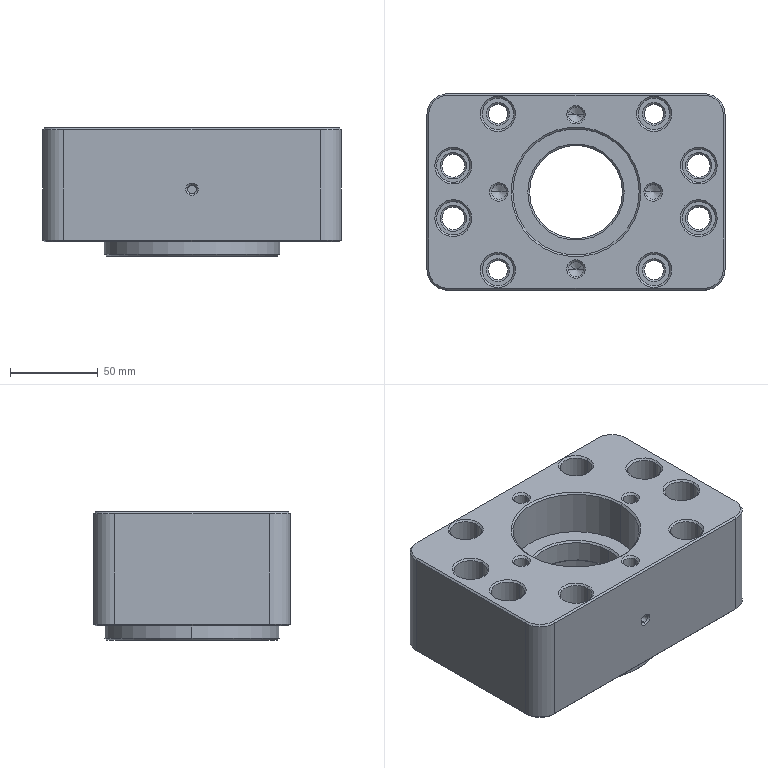NC program | NX | posted with a generic post | part box 170 x 112 x 73 mm
Lines 2870 to 3892 of 12198:
(ZLEVEL_PROFILE , TOOL : D26)
N5690 T16 M6
N5692 G54
N5694 G17 G0 G90 X100.366 Y-39.31 S1700 M3
N5696 G43 Z30. H16
N5698 Z-0.349
N5700 G94 G1 X99.295 Y-39.929 F1000.
N5702 G3 X97.997 Y-42.182 R2.6
N5704 G1 X97.998 Y-43.259 F1700.
N5706 X97.999 Y-44.01
N5708 G2 X97.948 Y-45.558 R44.459
N5710 X97.732 Y-47.632 R28.441
N5712 X97.189 Y-50.339 R30.228
N5714 X95.838 Y-54.175 R27.501
N5716 X92.835 Y-59.228 R26.139
N5718 X90.04 Y-62.3 R28.22
N5720 X88.018 Y-63.983 R28.318
N5722 X86.327 Y-65.148 R28.811
N5724 X83.495 Y-66.697 R27.897
N5726 X81.085 Y-67.653 R30.882
N5728 X77.976 Y-68.509 R29.143
N5730 X75.343 Y-68.886 R30.526
N5732 X73.425 Y-68.993 R29.282
N5734 G1 X73.01 Y-68.999
N5736 X72.259 Y-68.997
N5738 X71.182
N5740 G3 X68.93 Y-70.296 R2.6
N5742 G1 X68.311 Y-71.366
N5744 G0 Z30.
N5746 X100.367 Y-39.309
N5748 Z-0.699
N5750 G1 X99.295 Y-39.929 F1000.
N5752 G3 X97.997 Y-42.182 R2.6
N5754 G1 X97.998 Y-43.259 F1700.
N5756 X97.999 Y-44.01
N5758 G2 X97.948 Y-45.558 R41.97
N5760 X97.732 Y-47.632 R28.038
N5762 X97.183 Y-50.359 R29.625
N5764 X95.831 Y-54.19 R27.273
N5766 X94.533 Y-56.694 R26.82
N5768 X92.811 Y-59.258 R28.325
N5770 X90.033 Y-62.306 R28.036
N5772 X88.018 Y-63.983 R28.19
N5774 X86.328 Y-65.148 R28.641
N5776 X84.741 Y-66.068 R29.677
N5778 X82.981 Y-66.917 R27.561
N5780 X81.085 Y-67.653 R27.854
N5782 X77.947 Y-68.514 R28.668
N5784 X75.343 Y-68.886 R30.089
N5786 X73.425 Y-68.993 R28.844
N5788 G1 X73.01 Y-68.999
N5790 X72.259 Y-68.998
N5792 X71.182 Y-68.997
N5794 G3 X68.93 Y-70.296 R2.6
N5796 G1 X68.31 Y-71.367
N5798 G0 Z30.
N5800 X100.6 Y-39.169
N5802 Z-1.048
N5804 G1 X99.292 Y-39.928 F1000.
N5806 G3 X97.997 Y-42.182 R2.6
N5808 G1 X98. Y-43.617 F1700.
N5810 Y-44.
N5812 G2 X72.986 Y-69. R25.
N5814 G1 X72.617
N5816 X71.182 Y-68.997
N5818 G3 X68.928 Y-70.292 R2.6
N5820 G1 X68.169 Y-71.6
N5822 G0 Z30.
N5824 X100.6 Y-39.169
N5826 Z-1.398
N5828 G1 X99.292 Y-39.928 F1000.
N5830 G3 X97.997 Y-42.182 R2.6
N5832 G1 X98. Y-43.617 F1700.
N5834 Y-44.
N5836 G2 X72.986 Y-69. R25.
N5838 G1 X72.617
N5840 X71.182 Y-68.997
N5842 G3 X68.928 Y-70.292 R2.6
N5844 G1 X68.169 Y-71.6
N5846 G0 Z30.
N5848 X100.6 Y-39.169
N5850 Z-1.747
N5852 G1 X99.292 Y-39.928 F1000.
N5854 G3 X97.997 Y-42.182 R2.6
N5856 G1 X98. Y-43.617 F1700.
N5858 Y-44.
N5860 G2 X72.986 Y-69. R25.
N5862 G1 X72.617
N5864 X71.182 Y-68.997
N5866 G3 X68.928 Y-70.292 R2.6
N5868 G1 X68.169 Y-71.6
N5870 G0 Z30.
N5872 X100.6 Y-39.169
N5874 Z-2.097
N5876 G1 X99.292 Y-39.928 F1000.
N5878 G3 X97.997 Y-42.182 R2.6
N5880 G1 X98. Y-43.617 F1700.
N5882 Y-44.
N5884 G2 X72.986 Y-69. R25.
N5886 G1 X72.617
N5888 X71.182 Y-68.997
N5890 G3 X68.928 Y-70.292 R2.6
N5892 G1 X68.169 Y-71.6
N5894 G0 Z30.
N5896 X100.6 Y-39.169
N5898 Z-2.446
N5900 G1 X99.292 Y-39.928 F1000.
N5902 G3 X97.997 Y-42.182 R2.6
N5904 G1 X98. Y-43.617 F1700.
N5906 Y-44.
N5908 G2 X72.986 Y-69. R25.
N5910 G1 X72.617
N5912 X71.182 Y-68.997
N5914 G3 X68.928 Y-70.292 R2.6
N5916 G1 X68.169 Y-71.6
N5918 G0 Z30.
N5920 X100.6 Y-39.169
N5922 Z-2.796
N5924 G1 X99.292 Y-39.928 F1000.
N5926 G3 X97.997 Y-42.182 R2.6
N5928 G1 X98. Y-43.617 F1700.
N5930 Y-44.
N5932 G2 X72.986 Y-69. R25.
N5934 G1 X72.617
N5936 X71.182 Y-68.997
N5938 G3 X68.928 Y-70.292 R2.6
N5940 G1 X68.169 Y-71.6
N5942 G0 Z30.
N5944 X100.6 Y-39.169
N5946 Z-3.145
N5948 G1 X99.293 Y-39.928 F1000.
N5950 G3 X97.997 Y-42.182 R2.6
N5952 G1 X98. Y-43.617 F1700.
N5954 Y-44.
N5956 G2 X72.986 Y-69. R25.
N5958 G1 X72.617
N5960 X71.182 Y-68.997
N5962 G3 X68.928 Y-70.292 R2.6
N5964 G1 X68.169 Y-71.6
N5966 G0 Z30.
N5968 X100.6 Y-39.169
N5970 Z-3.495
N5972 G1 X99.293 Y-39.928 F1000.
N5974 G3 X97.997 Y-42.182 R2.6
N5976 G1 X98. Y-43.617 F1700.
N5978 Y-44.
N5980 G2 X72.986 Y-69. R25.
N5982 G1 X72.617
N5984 X71.182 Y-68.997
N5986 G3 X68.928 Y-70.292 R2.6
N5988 G1 X68.169 Y-71.6
N5990 G0 Z30.
N5992 X100.6 Y-39.17
N5994 Z-3.844
N5996 G1 X99.293 Y-39.928 F1000.
N5998 G3 X97.997 Y-42.182 R2.6
N6000 G1 X98. Y-43.617 F1700.
N6002 Y-44.
N6004 G2 X72.986 Y-69. R25.
N6006 G1 X72.617
N6008 X71.182 Y-68.997
N6010 G3 X68.928 Y-70.292 R2.6
N6012 G1 X68.169 Y-71.6
N6014 G0 Z30.
N6016 X100.6 Y-39.17
N6018 Z-4.194
N6020 G1 X99.293 Y-39.928 F1000.
N6022 G3 X97.997 Y-42.182 R2.6
N6024 G1 X98. Y-43.617 F1700.
N6026 Y-44.
N6028 G2 X72.986 Y-69. R25.
N6030 G1 X72.617
N6032 X71.182 Y-68.997
N6034 G3 X68.928 Y-70.292 R2.6
N6036 G1 X68.169 Y-71.6
N6038 G0 Z30.
N6040 X100.6 Y-39.17
N6042 Z-4.543
N6044 G1 X99.293 Y-39.928 F1000.
N6046 G3 X97.997 Y-42.182 R2.6
N6048 G1 X98. Y-43.617 F1700.
N6050 Y-44.
N6052 G2 X72.986 Y-69. R25.
N6054 G1 X72.617
N6056 X71.182 Y-68.997
N6058 G3 X68.928 Y-70.292 R2.6
N6060 G1 X68.169 Y-71.6
N6062 G0 Z30.
N6064 X100.6 Y-39.17
N6066 Z-4.892
N6068 G1 X99.293 Y-39.928 F1000.
N6070 G3 X97.997 Y-42.182 R2.6
N6072 G1 X98. Y-43.617 F1700.
N6074 Y-44.
N6076 G2 X72.986 Y-69. R25.
N6078 G1 X72.617
N6080 X71.182 Y-68.997
N6082 G3 X68.928 Y-70.292 R2.6
N6084 G1 X68.169 Y-71.6
N6086 G0 Z30.
N6088 X100.6 Y-39.17
N6090 Z-5.242
N6092 G1 X99.293 Y-39.928 F1000.
N6094 G3 X97.997 Y-42.182 R2.6
N6096 G1 X98. Y-43.617 F1700.
N6098 Y-44.
N6100 G2 X72.986 Y-69. R25.
N6102 G1 X72.617
N6104 X71.182 Y-68.997
N6106 G3 X68.928 Y-70.292 R2.6
N6108 G1 X68.169 Y-71.6
N6110 G0 Z30.
N6112 X100.6 Y-39.17
N6114 Z-5.591
N6116 G1 X99.293 Y-39.928 F1000.
N6118 G3 X97.997 Y-42.182 R2.6
N6120 G1 X98. Y-43.617 F1700.
N6122 Y-44.
N6124 G2 X72.986 Y-69. R25.
N6126 G1 X72.617
N6128 X71.182 Y-68.997
N6130 G3 X68.928 Y-70.292 R2.6
N6132 G1 X68.169 Y-71.6
N6134 G0 Z30.
N6136 X100.6 Y-39.17
N6138 Z-5.941
N6140 G1 X99.293 Y-39.928 F1000.
N6142 G3 X97.997 Y-42.182 R2.6
N6144 G1 X98. Y-43.617 F1700.
N6146 Y-44.
N6148 G2 X72.986 Y-69. R25.
N6150 G1 X72.617
N6152 X71.182 Y-68.997
N6154 G3 X68.928 Y-70.292 R2.6
N6156 G1 X68.169 Y-71.6
N6158 G0 Z30.
N6160 X100.6 Y-39.17
N6162 Z-6.29
N6164 G1 X99.293 Y-39.928 F1000.
N6166 G3 X97.997 Y-42.182 R2.6
N6168 G1 X98. Y-43.617 F1700.
N6170 Y-44.
N6172 G2 X72.986 Y-69. R25.
N6174 G1 X72.617
N6176 X71.182 Y-68.997
N6178 G3 X68.928 Y-70.293 R2.6
N6180 G1 X68.169 Y-71.6
N6182 G0 Z30.
N6184 X100.6 Y-39.17
N6186 Z-6.64
N6188 G1 X99.293 Y-39.928 F1000.
N6190 G3 X97.997 Y-42.182 R2.6
N6192 G1 X98. Y-43.617 F1700.
N6194 Y-44.
N6196 G2 X72.986 Y-69. R25.
N6198 G1 X72.617
N6200 X71.182 Y-68.997
N6202 G3 X68.928 Y-70.293 R2.6
N6204 G1 X68.169 Y-71.6
N6206 G0 Z30.
N6208 X100.6 Y-39.17
N6210 Z-6.989
N6212 G1 X99.293 Y-39.928 F1000.
N6214 G3 X97.997 Y-42.182 R2.6
N6216 G1 X98. Y-43.617 F1700.
N6218 Y-44.
N6220 G2 X72.986 Y-69. R25.
N6222 G1 X72.617
N6224 X71.182 Y-68.997
N6226 G3 X68.928 Y-70.293 R2.6
N6228 G1 X68.169 Y-71.6
N6230 G0 Z30.
N6232 X100.6 Y-39.17
N6234 Z-7.339
N6236 G1 X99.293 Y-39.928 F1000.
N6238 G3 X97.997 Y-42.182 R2.6
N6240 G1 X98. Y-43.617 F1700.
N6242 Y-44.
N6244 G2 X72.986 Y-69. R25.
N6246 G1 X72.617
N6248 X71.182 Y-68.997
N6250 G3 X68.928 Y-70.293 R2.6
N6252 G1 X68.169 Y-71.6
N6254 G0 Z30.
N6256 X100.6 Y-39.17
N6258 Z-7.688
N6260 G1 X99.293 Y-39.928 F1000.
N6262 G3 X97.997 Y-42.182 R2.6
N6264 G1 X98. Y-43.617 F1700.
N6266 Y-44.
N6268 G2 X72.986 Y-69. R25.
N6270 G1 X72.617
N6272 X71.182 Y-68.997
N6274 G3 X68.928 Y-70.293 R2.6
N6276 G1 X68.17 Y-71.6
N6278 G0 Z30.
N6280 X100.6 Y-39.17
N6282 Z-8.038
N6284 G1 X99.293 Y-39.928 F1000.
N6286 G3 X97.997 Y-42.182 R2.6
N6288 G1 X98. Y-43.617 F1700.
N6290 Y-44.
N6292 G2 X72.986 Y-69. R25.
N6294 G1 X72.617
N6296 X71.182 Y-68.997
N6298 G3 X68.928 Y-70.293 R2.6
N6300 G1 X68.17 Y-71.6
N6302 G0 Z30.
N6304 X100.6 Y-39.17
N6306 Z-8.387
N6308 G1 X99.293 Y-39.928 F1000.
N6310 G3 X97.997 Y-42.182 R2.6
N6312 G1 X98. Y-43.617 F1700.
N6314 Y-44.
N6316 G2 X72.986 Y-69. R25.
N6318 G1 X72.617
N6320 X71.182 Y-68.997
N6322 G3 X68.928 Y-70.293 R2.6
N6324 G1 X68.17 Y-71.6
N6326 G0 Z30.
N6328 X100.6 Y-39.17
N6330 Z-8.737
N6332 G1 X99.293 Y-39.928 F1000.
N6334 G3 X97.997 Y-42.182 R2.6
N6336 G1 X98. Y-43.617 F1700.
N6338 Y-44.
N6340 G2 X72.986 Y-69. R25.
N6342 G1 X72.617
N6344 X71.182 Y-68.997
N6346 G3 X68.928 Y-70.293 R2.6
N6348 G1 X68.17 Y-71.6
N6350 G0 Z30.
N6352 X100.6 Y-39.17
N6354 Z-9.086
N6356 G1 X99.293 Y-39.928 F1000.
N6358 G3 X97.997 Y-42.182 R2.6
N6360 G1 X98. Y-43.617 F1700.
N6362 Y-44.
N6364 G2 X72.986 Y-69. R25.
N6366 G1 X72.617
N6368 X71.182 Y-68.997
N6370 G3 X68.928 Y-70.293 R2.6
N6372 G1 X68.17 Y-71.6
N6374 G0 Z30.
N6376 X100.6 Y-39.17
N6378 Z-9.435
N6380 G1 X99.293 Y-39.928 F1000.
N6382 G3 X97.997 Y-42.182 R2.6
N6384 G1 X98. Y-43.617 F1700.
N6386 Y-44.
N6388 G2 X72.986 Y-69. R25.
N6390 G1 X72.617
N6392 X71.182 Y-68.997
N6394 G3 X68.928 Y-70.293 R2.6
N6396 G1 X68.17 Y-71.6
N6398 G0 Z30.
N6400 X100.6 Y-39.171
N6402 Z-9.785
N6404 G1 X99.293 Y-39.928 F1000.
N6406 G3 X97.997 Y-42.182 R2.6
N6408 G1 X98. Y-43.617 F1700.
N6410 Y-44.
N6412 G2 X72.986 Y-69. R25.
N6414 G1 X72.617
N6416 X71.182 Y-68.997
N6418 G3 X68.928 Y-70.293 R2.6
N6420 G1 X68.17 Y-71.6
N6422 G0 Z30.
N6424 X100.6 Y-39.171
N6426 Z-10.134
N6428 G1 X99.293 Y-39.928 F1000.
N6430 G3 X97.997 Y-42.182 R2.6
N6432 G1 X98. Y-43.617 F1700.
N6434 Y-44.
N6436 G2 X72.986 Y-69. R25.
N6438 G1 X72.617
N6440 X71.182 Y-68.997
N6442 G3 X68.928 Y-70.293 R2.6
N6444 G1 X68.17 Y-71.6
N6446 G0 Z30.
N6448 X100.6 Y-39.171
N6450 Z-10.484
N6452 G1 X99.293 Y-39.928 F1000.
N6454 G3 X97.997 Y-42.182 R2.6
N6456 G1 X98. Y-43.617 F1700.
N6458 Y-44.
N6460 G2 X72.986 Y-69. R25.
N6462 G1 X72.617
N6464 X71.182 Y-68.997
N6466 G3 X68.928 Y-70.293 R2.6
N6468 G1 X68.17 Y-71.6
N6470 G0 Z30.
N6472 X100.6 Y-39.171
N6474 Z-10.833
N6476 G1 X99.293 Y-39.928 F1000.
N6478 G3 X97.997 Y-42.182 R2.6
N6480 G1 X98. Y-43.617 F1700.
N6482 Y-44.
N6484 G2 X72.986 Y-69. R25.
N6486 G1 X72.617
N6488 X71.182 Y-68.997
N6490 G3 X68.928 Y-70.293 R2.6
N6492 G1 X68.17 Y-71.6
N6494 G0 Z30.
N6496 X100.6 Y-39.171
N6498 Z-11.183
N6500 G1 X99.293 Y-39.928 F1000.
N6502 G3 X97.997 Y-42.182 R2.6
N6504 G1 X98. Y-43.617 F1700.
N6506 Y-44.
N6508 G2 X72.986 Y-69. R25.
N6510 G1 X72.617
N6512 X71.182 Y-68.997
N6514 G3 X68.928 Y-70.293 R2.6
N6516 G1 X68.17 Y-71.6
N6518 G0 Z30.
N6520 X100.6 Y-39.171
N6522 Z-11.532
N6524 G1 X99.294 Y-39.928 F1000.
N6526 G3 X97.997 Y-42.182 R2.6
N6528 G1 X98. Y-43.617 F1700.
N6530 Y-44.
N6532 G2 X72.986 Y-69. R25.
N6534 G1 X72.617
N6536 X71.182 Y-68.997
N6538 G3 X68.928 Y-70.293 R2.6
N6540 G1 X68.17 Y-71.6
N6542 G0 Z30.
N6544 X100.6 Y-39.171
N6546 Z-11.882
N6548 G1 X99.294 Y-39.928 F1000.
N6550 G3 X97.997 Y-42.182 R2.6
N6552 G1 X98. Y-43.617 F1700.
N6554 Y-44.
N6556 G2 X72.986 Y-69. R25.
N6558 G1 X72.617
N6560 X71.182 Y-68.997
N6562 G3 X68.928 Y-70.293 R2.6
N6564 G1 X68.17 Y-71.6
N6566 G0 Z30.
N6568 X100.6 Y-39.171
N6570 Z-12.231
N6572 G1 X99.294 Y-39.928 F1000.
N6574 G3 X97.998 Y-42.182 R2.6
N6576 G1 X98. Y-43.617 F1700.
N6578 Y-44.
N6580 G2 X72.986 Y-69. R25.
N6582 G1 X72.617
N6584 X71.182 Y-68.997
N6586 G3 X68.928 Y-70.293 R2.6
N6588 G1 X68.17 Y-71.6
N6590 G0 Z30.
N6592 X100.6 Y-39.171
N6594 Z-12.581
N6596 G1 X99.294 Y-39.928 F1000.
N6598 G3 X97.998 Y-42.182 R2.6
N6600 G1 X98. Y-43.617 F1700.
N6602 Y-44.
N6604 G2 X72.986 Y-69. R25.
N6606 G1 X72.617
N6608 X71.182 Y-68.997
N6610 G3 X68.928 Y-70.293 R2.6
N6612 G1 X68.17 Y-71.6
N6614 G0 Z30.
N6616 X100.6 Y-39.171
N6618 Z-12.93
N6620 G1 X99.294 Y-39.928 F1000.
N6622 G3 X97.998 Y-42.182 R2.6
N6624 G1 X98. Y-43.617 F1700.
N6626 Y-44.
N6628 G2 X72.986 Y-69. R25.
N6630 G1 X72.617
N6632 X71.182 Y-68.997
N6634 G3 X68.928 Y-70.293 R2.6
N6636 G1 X68.17 Y-71.6
N6638 G0 Z30.
N6640 X100.6 Y-39.171
N6642 Z-13.28
N6644 G1 X99.294 Y-39.928 F1000.
N6646 G3 X97.998 Y-42.182 R2.6
N6648 G1 X98. Y-43.617 F1700.
N6650 Y-44.
N6652 G2 X72.986 Y-69. R25.
N6654 G1 X72.617
N6656 X71.182 Y-68.997
N6658 G3 X68.928 Y-70.293 R2.6
N6660 G1 X68.17 Y-71.6
N6662 G0 Z30.
N6664 X100.6 Y-39.171
N6666 Z-13.629
N6668 G1 X99.294 Y-39.928 F1000.
N6670 G3 X97.998 Y-42.182 R2.6
N6672 G1 X98. Y-43.617 F1700.
N6674 Y-44.
N6676 G2 X72.986 Y-69. R25.
N6678 G1 X72.617
N6680 X71.182 Y-68.997
N6682 G3 X68.928 Y-70.293 R2.6
N6684 G1 X68.17 Y-71.6
N6686 G0 Z30.
N6688 X100.6 Y-39.171
N6690 Z-13.978
N6692 G1 X99.294 Y-39.928 F1000.
N6694 G3 X97.998 Y-42.182 R2.6
N6696 G1 X98. Y-43.617 F1700.
N6698 Y-44.
N6700 G2 X72.986 Y-69. R25.
N6702 G1 X72.617
N6704 X71.182 Y-68.997
N6706 G3 X68.928 Y-70.293 R2.6
N6708 G1 X68.17 Y-71.6
N6710 G0 Z30.
N6712 X100.6 Y-39.171
N6714 Z-14.328
N6716 G1 X99.294 Y-39.928 F1000.
N6718 G3 X97.998 Y-42.182 R2.6
N6720 G1 X98. Y-43.617 F1700.
N6722 Y-44.
N6724 G2 X72.986 Y-69. R25.
N6726 G1 X72.617
N6728 X71.182 Y-68.997
N6730 G3 X68.928 Y-70.293 R2.6
N6732 G1 X68.17 Y-71.6
N6734 G0 Z30.
N6736 X100.6 Y-39.171
N6738 Z-14.677
N6740 G1 X99.294 Y-39.928 F1000.
N6742 G3 X97.998 Y-42.182 R2.6
N6744 G1 X98. Y-43.617 F1700.
N6746 Y-44.
N6748 G2 X72.986 Y-69. R25.
N6750 G1 X72.617
N6752 X71.182 Y-68.997
N6754 G3 X68.928 Y-70.293 R2.6
N6756 G1 X68.17 Y-71.6
N6758 G0 Z30.
N6760 X100.6 Y-39.171
N6762 Z-15.027
N6764 G1 X99.294 Y-39.928 F1000.
N6766 G3 X97.998 Y-42.182 R2.6
N6768 G1 X98. Y-43.617 F1700.
N6770 Y-44.
N6772 G2 X72.986 Y-69. R25.
N6774 G1 X72.617
N6776 X71.182 Y-68.997
N6778 G3 X68.928 Y-70.293 R2.6
N6780 G1 X68.17 Y-71.6
N6782 G0 Z30.
N6784 X100.6 Y-39.171
N6786 Z-15.376
N6788 G1 X99.294 Y-39.928 F1000.
N6790 G3 X97.998 Y-42.182 R2.6
N6792 G1 X98. Y-43.617 F1700.
N6794 Y-44.
N6796 G2 X72.986 Y-69. R25.
N6798 G1 X72.617
N6800 X71.182 Y-68.997
N6802 G3 X68.928 Y-70.293 R2.6
N6804 G1 X68.17 Y-71.6
N6806 G0 Z30.
N6808 X100.6 Y-39.172
N6810 Z-15.726
N6812 G1 X99.294 Y-39.928 F1000.
N6814 G3 X97.998 Y-42.182 R2.6
N6816 G1 X98. Y-43.617 F1700.
N6818 Y-44.
N6820 G2 X72.986 Y-69. R25.
N6822 G1 X72.617
N6824 X71.182 Y-68.997
N6826 G3 X68.928 Y-70.293 R2.6
N6828 G1 X68.17 Y-71.6
N6830 G0 Z30.
N6832 X100.6 Y-39.172
N6834 Z-16.075
N6836 G1 X99.294 Y-39.928 F1000.
N6838 G3 X97.998 Y-42.182 R2.6
N6840 G1 X98. Y-43.617 F1700.
N6842 Y-44.
N6844 G2 X72.986 Y-69. R25.
N6846 G1 X72.617
N6848 X71.182 Y-68.997
N6850 G3 X68.928 Y-70.293 R2.6
N6852 G1 X68.17 Y-71.6
N6854 G0 Z30.
N6856 X100.6 Y-39.172
N6858 Z-16.425
N6860 G1 X99.294 Y-39.928 F1000.
N6862 G3 X97.998 Y-42.182 R2.6
N6864 G1 X98. Y-43.617 F1700.
N6866 Y-44.
N6868 G2 X72.986 Y-69. R25.
N6870 G1 X72.617
N6872 X71.182 Y-68.997
N6874 G3 X68.928 Y-70.293 R2.6
N6876 G1 X68.17 Y-71.6
N6878 G0 Z30.
N6880 X100.6 Y-39.172
N6882 Z-16.774
N6884 G1 X99.294 Y-39.928 F1000.
N6886 G3 X97.998 Y-42.182 R2.6
N6888 G1 X98. Y-43.617 F1700.
N6890 Y-44.
N6892 G2 X72.986 Y-69. R25.
N6894 G1 X72.617
N6896 X71.182 Y-68.997
N6898 G3 X68.928 Y-70.293 R2.6
N6900 G1 X68.17 Y-71.6
N6902 G0 Z30.
N6904 X100.6 Y-39.172
N6906 Z-17.124
N6908 G1 X99.294 Y-39.928 F1000.
N6910 G3 X97.998 Y-42.182 R2.6
N6912 G1 X98. Y-43.617 F1700.
N6914 Y-44.
N6916 G2 X72.986 Y-69. R25.
N6918 G1 X72.617
N6920 X71.182 Y-68.997
N6922 G3 X68.928 Y-70.293 R2.6
N6924 G1 X68.17 Y-71.6
N6926 G0 Z30.
N6928 X100.6 Y-39.172
N6930 Z-17.473
N6932 G1 X99.294 Y-39.928 F1000.
N6934 G3 X97.998 Y-42.182 R2.6
N6936 G1 X98. Y-43.617 F1700.
N6938 Y-44.
N6940 G2 X72.986 Y-69. R25.
N6942 G1 X72.617
N6944 X71.182 Y-68.997
N6946 G3 X68.928 Y-70.293 R2.6
N6948 G1 X68.17 Y-71.6
N6950 G0 Z30.
N6952 X100.6 Y-39.172
N6954 Z-17.823
N6956 G1 X99.294 Y-39.928 F1000.
N6958 G3 X97.998 Y-42.182 R2.6
N6960 G1 X98. Y-43.617 F1700.
N6962 Y-44.
N6964 G2 X72.986 Y-69. R25.
N6966 G1 X72.617
N6968 X71.182 Y-68.997
N6970 G3 X68.928 Y-70.293 R2.6
N6972 G1 X68.17 Y-71.6
N6974 G0 Z30.
N6976 X100.6 Y-39.172
N6978 Z-18.172
N6980 G1 X99.294 Y-39.928 F1000.
N6982 G3 X97.998 Y-42.182 R2.6
N6984 G1 X98. Y-43.617 F1700.
N6986 Y-44.
N6988 G2 X72.986 Y-69. R25.
N6990 G1 X72.617
N6992 X71.182 Y-68.997
N6994 G3 X68.928 Y-70.293 R2.6
N6996 G1 X68.171 Y-71.6
N6998 G0 Z30.
N7000 X100.6 Y-39.172
N7002 Z-18.522
N7004 G1 X99.294 Y-39.928 F1000.
N7006 G3 X97.998 Y-42.182 R2.6
N7008 G1 X98. Y-43.617 F1700.
N7010 Y-44.
N7012 G2 X72.986 Y-69. R25.
N7014 G1 X72.617
N7016 X71.182 Y-68.997
N7018 G3 X68.928 Y-70.293 R2.6
N7020 G1 X68.171 Y-71.6
N7022 G0 Z30.
N7024 X100.6 Y-39.172
N7026 Z-18.871
N7028 G1 X99.294 Y-39.928 F1000.
N7030 G3 X97.998 Y-42.182 R2.6
N7032 G1 X98. Y-43.617 F1700.
N7034 Y-44.
N7036 G2 X72.986 Y-69. R25.
N7038 G1 X72.617
N7040 X71.182 Y-68.997
N7042 G3 X68.928 Y-70.293 R2.6
N7044 G1 X68.171 Y-71.6
N7046 G0 Z30.
N7048 X100.6 Y-39.172
N7050 Z-19.22
N7052 G1 X99.294 Y-39.928 F1000.
N7054 G3 X97.998 Y-42.182 R2.6
N7056 G1 X98. Y-43.617 F1700.
N7058 Y-44.
N7060 G2 X72.986 Y-69. R25.
N7062 G1 X72.617
N7064 X71.182 Y-68.997
N7066 G3 X68.928 Y-70.293 R2.6
N7068 G1 X68.171 Y-71.6
N7070 G0 Z30.
N7072 X100.6 Y-39.172
N7074 Z-19.57
N7076 G1 X99.294 Y-39.929 F1000.
N7078 G3 X97.998 Y-42.182 R2.6
N7080 G1 X98. Y-43.617 F1700.
N7082 Y-44.
N7084 G2 X72.986 Y-69. R25.
N7086 G1 X72.617
N7088 X71.182 Y-68.997
N7090 G3 X68.928 Y-70.293 R2.6
N7092 G1 X68.171 Y-71.6
N7094 G0 Z30.
N7096 X100.6 Y-39.172
N7098 Z-19.919
N7100 G1 X99.295 Y-39.929 F1000.
N7102 G3 X97.998 Y-42.182 R2.6
N7104 G1 X98. Y-43.617 F1700.
N7106 Y-44.
N7108 G2 X72.986 Y-69. R25.
N7110 G1 X72.617
N7112 X71.182 Y-68.997
N7114 G3 X68.928 Y-70.293 R2.6
N7116 G1 X68.171 Y-71.6
N7118 G0 Z30.
N7120 X100.6 Y-39.172
N7122 Z-20.269
N7124 G1 X99.295 Y-39.929 F1000.
N7126 G3 X97.998 Y-42.182 R2.6
N7128 G1 X98. Y-43.617 F1700.
N7130 Y-44.
N7132 G2 X72.986 Y-69. R25.
N7134 G1 X72.617
N7136 X71.182 Y-68.997
N7138 G3 X68.928 Y-70.293 R2.6
N7140 G1 X68.171 Y-71.6
N7142 G0 Z30.
N7144 X100.6 Y-39.172
N7146 Z-20.618
N7148 G1 X99.295 Y-39.929 F1000.
N7150 G3 X97.998 Y-42.182 R2.6
N7152 G1 X98. Y-43.617 F1700.
N7154 Y-44.
N7156 G2 X72.986 Y-69. R25.
N7158 G1 X72.617
N7160 X71.182 Y-68.997
N7162 G3 X68.928 Y-70.293 R2.6
N7164 G1 X68.171 Y-71.6
N7166 G0 Z30.
N7168 X100.6 Y-39.172
N7170 Z-20.968
N7172 G1 X99.295 Y-39.929 F1000.
N7174 G3 X97.998 Y-42.182 R2.6
N7176 G1 X98. Y-43.617 F1700.
N7178 Y-44.
N7180 G2 X72.986 Y-69. R25.
N7182 G1 X72.617
N7184 X71.182 Y-68.997
N7186 G3 X68.928 Y-70.293 R2.6
N7188 G1 X68.171 Y-71.6
N7190 G0 Z30.
N7192 X100.6 Y-39.172
N7194 Z-21.317
N7196 G1 X99.295 Y-39.929 F1000.
N7198 G3 X97.998 Y-42.182 R2.6
N7200 G1 X98. Y-43.617 F1700.
N7202 Y-44.
N7204 G2 X72.986 Y-69. R25.
N7206 G1 X72.617
N7208 X71.182 Y-68.997
N7210 G3 X68.928 Y-70.294 R2.6
N7212 G1 X68.171 Y-71.6
N7214 G0 Z30.
N7216 X100.6 Y-39.172
N7218 Z-21.667
N7220 G1 X99.295 Y-39.929 F1000.
N7222 G3 X97.998 Y-42.182 R2.6
N7224 G1 X98. Y-43.617 F1700.
N7226 Y-44.
N7228 G2 X72.986 Y-69. R25.
N7230 G1 X72.617
N7232 X71.182 Y-68.997
N7234 G3 X68.928 Y-70.294 R2.6
N7236 G1 X68.171 Y-71.6
N7238 G0 Z30.
N7240 X100.6 Y-39.173
N7242 Z-22.016
N7244 G1 X99.295 Y-39.929 F1000.
N7246 G3 X97.998 Y-42.182 R2.6
N7248 G1 X98. Y-43.617 F1700.
N7250 Y-44.
N7252 G2 X72.986 Y-69. R25.
N7254 G1 X72.617
N7256 X71.182 Y-68.997
N7258 G3 X68.928 Y-70.294 R2.6
N7260 G1 X68.171 Y-71.6
N7262 G0 Z30.
N7264 X100.6 Y-39.173
N7266 Z-22.366
N7268 G1 X99.295 Y-39.929 F1000.
N7270 G3 X97.998 Y-42.182 R2.6
N7272 G1 X98. Y-43.617 F1700.
N7274 Y-44.
N7276 G2 X72.986 Y-69. R25.
N7278 G1 X72.617
N7280 X71.182 Y-68.998
N7282 G3 X68.928 Y-70.294 R2.6
N7284 G1 X68.171 Y-71.6
N7286 G0 Z30.
N7288 X100.6 Y-39.173
N7290 Z-22.715
N7292 G1 X99.295 Y-39.929 F1000.
N7294 G3 X97.998 Y-42.182 R2.6
N7296 G1 X98. Y-43.617 F1700.
N7298 Y-44.
N7300 G2 X72.986 Y-69. R25.
N7302 G1 X72.617
N7304 X71.182 Y-68.998
N7306 G3 X68.928 Y-70.294 R2.6
N7308 G1 X68.171 Y-71.6
N7310 G0 Z30.
N7312 X100.6 Y-39.173
N7314 Z-23.065
N7316 G1 X99.295 Y-39.929 F1000.
N7318 G3 X97.998 Y-42.182 R2.6
N7320 G1 X98. Y-43.617 F1700.
N7322 Y-44.
N7324 G2 X72.986 Y-69. R25.
N7326 G1 X72.617
N7328 X71.182 Y-68.998
N7330 G3 X68.928 Y-70.294 R2.6
N7332 G1 X68.171 Y-71.6
N7334 G0 Z30.
N7336 X100.6 Y-39.173
N7338 Z-23.414
N7340 G1 X99.295 Y-39.929 F1000.
N7342 G3 X97.998 Y-42.182 R2.6
N7344 G1 X98. Y-43.617 F1700.
N7346 Y-44.
N7348 G2 X72.986 Y-69. R25.
N7350 G1 X72.617
N7352 X71.182 Y-68.998
N7354 G3 X68.928 Y-70.294 R2.6
N7356 G1 X68.171 Y-71.6
N7358 G0 Z30.
N7360 X100.6 Y-39.173
N7362 Z-23.763
N7364 G1 X99.295 Y-39.929 F1000.
N7366 G3 X97.998 Y-42.182 R2.6
N7368 G1 X98. Y-43.617 F1700.
N7370 Y-44.
N7372 G2 X72.986 Y-69. R25.
N7374 G1 X72.617
N7376 X71.182 Y-68.998
N7378 G3 X68.928 Y-70.294 R2.6
N7380 G1 X68.171 Y-71.6
N7382 G0 Z30.
N7384 X100.6 Y-39.173
N7386 Z-24.113
N7388 G1 X99.295 Y-39.929 F1000.
N7390 G3 X97.998 Y-42.182 R2.6
N7392 G1 X98. Y-43.617 F1700.
N7394 Y-44.
N7396 G2 X72.986 Y-69. R25.
N7398 G1 X72.617
N7400 X71.182 Y-68.998
N7402 G3 X68.928 Y-70.294 R2.6
N7404 G1 X68.171 Y-71.6
N7406 G0 Z30.
N7408 X100.6 Y-39.173
N7410 Z-24.462
N7412 G1 X99.295 Y-39.929 F1000.
N7414 G3 X97.998 Y-42.182 R2.6
N7416 G1 X98. Y-43.617 F1700.
N7418 Y-44.
N7420 G2 X72.986 Y-69. R25.
N7422 G1 X72.617
N7424 X71.182 Y-68.998
N7426 G3 X68.928 Y-70.294 R2.6
N7428 G1 X68.171 Y-71.6
N7430 G0 Z30.
N7432 X100.6 Y-39.173
N7434 Z-24.812
N7436 G1 X99.295 Y-39.929 F1000.
N7438 G3 X97.998 Y-42.182 R2.6
N7440 G1 X98. Y-43.617 F1700.
N7442 Y-44.
N7444 G2 X72.986 Y-69. R25.
N7446 G1 X72.617
N7448 X71.182 Y-68.998
N7450 G3 X68.928 Y-70.294 R2.6
N7452 G1 X68.171 Y-71.6
N7454 G0 Z30.
N7456 X100.6 Y-39.173
N7458 Z-25.161
N7460 G1 X99.295 Y-39.929 F1000.
N7462 G3 X97.998 Y-42.182 R2.6
N7464 G1 X98. Y-43.617 F1700.
N7466 Y-44.
N7468 G2 X72.986 Y-69. R25.
N7470 G1 X72.617
N7472 X71.182 Y-68.998
N7474 G3 X68.928 Y-70.294 R2.6
N7476 G1 X68.171 Y-71.6
N7478 G0 Z30.
N7480 X100.6 Y-39.173
N7482 Z-25.511
N7484 G1 X99.295 Y-39.929 F1000.
N7486 G3 X97.998 Y-42.182 R2.6
N7488 G1 X98. Y-43.617 F1700.
N7490 Y-44.
N7492 G2 X72.986 Y-69. R25.
N7494 G1 X72.617
N7496 X71.182 Y-68.998
N7498 G3 X68.928 Y-70.294 R2.6
N7500 G1 X68.171 Y-71.6
N7502 G0 Z30.
N7504 X100.6 Y-39.173
N7506 Z-25.86
N7508 G1 X99.295 Y-39.929 F1000.
N7510 G3 X97.998 Y-42.182 R2.6
N7512 G1 X98. Y-43.617 F1700.
N7514 Y-44.
N7516 G2 X72.986 Y-69. R25.
N7518 G1 X72.617
N7520 X71.182 Y-68.998
N7522 G3 X68.928 Y-70.294 R2.6
N7524 G1 X68.171 Y-71.6
N7526 G0 Z30.
N7528 X100.6 Y-39.173
N7530 Z-26.21
N7532 G1 X99.295 Y-39.929 F1000.
N7534 G3 X97.998 Y-42.182 R2.6
N7536 G1 X98. Y-43.617 F1700.
N7538 Y-44.
N7540 G2 X72.986 Y-69. R25.
N7542 G1 X72.617
N7544 X71.182 Y-68.998
N7546 G3 X68.928 Y-70.294 R2.6
N7548 G1 X68.171 Y-71.6
N7550 G0 Z30.
N7552 X100.6 Y-39.173
N7554 Z-26.559
N7556 G1 X99.295 Y-39.929 F1000.
N7558 G3 X97.998 Y-42.182 R2.6
N7560 G1 X98. Y-43.617 F1700.
N7562 Y-44.
N7564 G2 X72.986 Y-69. R25.
N7566 G1 X72.617
N7568 X71.182 Y-68.998
N7570 G3 X68.928 Y-70.294 R2.6
N7572 G1 X68.171 Y-71.6
N7574 G0 Z30.
N7576 X100.6 Y-39.173
N7578 Z-26.909
N7580 G1 X99.295 Y-39.929 F1000.
N7582 G3 X97.998 Y-42.182 R2.6
N7584 G1 X98. Y-43.617 F1700.
N7586 Y-44.
N7588 G2 X72.986 Y-69. R25.
N7590 G1 X72.617
N7592 X71.182 Y-68.998
N7594 G3 X68.928 Y-70.294 R2.6
N7596 G1 X68.171 Y-71.6
N7598 G0 Z30.
N7600 X100.6 Y-39.173
N7602 Z-27.258
N7604 G1 X99.295 Y-39.929 F1000.
N7606 G3 X97.998 Y-42.182 R2.6
N7608 G1 X98. Y-43.617 F1700.
N7610 Y-44.
N7612 G2 X72.986 Y-69. R25.
N7614 G1 X72.617
N7616 X71.182 Y-68.998
N7618 G3 X68.928 Y-70.294 R2.6
N7620 G1 X68.171 Y-71.6
N7622 G0 Z30.
N7624 X100.6 Y-39.173
N7626 Z-27.608
N7628 G1 X99.295 Y-39.929 F1000.
N7630 G3 X97.998 Y-42.182 R2.6
N7632 G1 X98. Y-43.617 F1700.
N7634 Y-44.
N7636 G2 X72.986 Y-69. R25.
N7638 G1 X72.617
N7640 X71.182 Y-68.998
N7642 G3 X68.928 Y-70.294 R2.6
N7644 G1 X68.171 Y-71.6
N7646 G0 Z30.
N7648 X100.6 Y-39.174
N7650 Z-27.957
N7652 G1 X99.295 Y-39.929 F1000.
N7654 G3 X97.998 Y-42.182 R2.6
N7656 G1 X98. Y-43.617 F1700.
N7658 Y-44.
N7660 G2 X72.986 Y-69. R25.
N7662 G1 X72.617
N7664 X71.182 Y-68.998
N7666 G3 X68.928 Y-70.294 R2.6
N7668 G1 X68.171 Y-71.6
N7670 G0 Z30.
N7672 X100.6 Y-39.174
N7674 Z-28.306
N7676 G1 X99.296 Y-39.929 F1000.
N7678 G3 X97.998 Y-42.182 R2.6
N7680 G1 X98. Y-43.617 F1700.
N7682 Y-44.
N7684 G2 X72.986 Y-69. R25.
N7686 G1 X72.617
N7688 X71.182 Y-68.998
N7690 G3 X68.928 Y-70.294 R2.6
N7692 G1 X68.171 Y-71.6
N7694 G0 Z30.
N7696 X100.6 Y-39.174
N7698 Z-28.656
N7700 G1 X99.296 Y-39.929 F1000.
N7702 G3 X97.998 Y-42.182 R2.6
N7704 G1 X98. Y-43.617 F1700.
N7706 Y-44.
N7708 G2 X72.986 Y-69. R25.
N7710 G1 X72.617
N7712 X71.182 Y-68.998
N7714 G3 X68.928 Y-70.294 R2.6
N7716 G1 X68.171 Y-71.6
N7718 G0 Z30.
N7720 X100.6 Y-39.174
N7722 Z-29.005
N7724 G1 X99.296 Y-39.929 F1000.
N7726 G3 X97.998 Y-42.182 R2.6
N7728 G1 X98. Y-43.617 F1700.